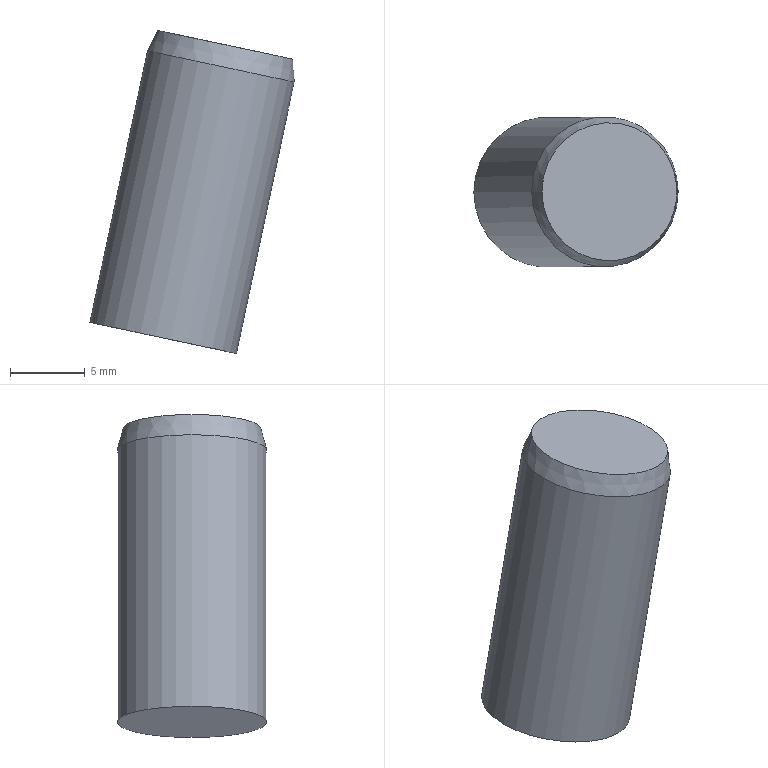Part | STEP file | 8903-XA820 dowel pin (φ8×20) | 1 solid | 4 faces | box 13.634 x 10 x 21.56 mm | volume 1562 mm3 | plane 2 | cone 1 | cylinder 1 | commonest cylinder face diameters 10 x1
STEP:
#1=CARTESIAN_POINT('',(0.,0.,0.));
#2=DIRECTION('',(0.,0.,1.));
#3=DIRECTION('',(1.,0.,0.));
#4=AXIS2_PLACEMENT_3D('',#1,#2,#3);
#5=CARTESIAN_POINT('',(2066.837,-149.5,-389.927));
#6=VERTEX_POINT('',#5);
#7=CARTESIAN_POINT('',(2071.342,-149.5,-390.885));
#8=DIRECTION('',(0.2079,0.,0.9781));
#9=DIRECTION('',(0.9781,0.,-0.2079));
#10=AXIS2_PLACEMENT_3D('',#7,#8,#9);
#11=CIRCLE('',#10,4.607);
#12=CARTESIAN_POINT('',(2069.596,-149.5,-390.514));
#13=DIRECTION('',(0.2079,0.,0.9781));
#14=DIRECTION('',(0.,1.,0.));
#15=AXIS2_PLACEMENT_3D('',#12,#13,#14);
#16=PLANE('',#15);
#17=CARTESIAN_POINT('',(0.,-1.786));
#18=DIRECTION('',(0.,-1.));
#19=AXIS2_PLACEMENT_2D('',#17,#18);
#20=CIRCLE('',#19,4.607);
#21=(GEOMETRIC_REPRESENTATION_CONTEXT(2)PARAMETRIC_REPRESENTATION_CONTEXT()REPRESENTATION_CONTEXT('',''));
#22=DEFINITIONAL_REPRESENTATION('',(#20),#21);
#23=PCURVE('',#16,#22);
#24=CARTESIAN_POINT('',(2071.23,-149.5,-391.414));
#25=DIRECTION('',(-0.2079,0.,-0.9781));
#26=DIRECTION('',(-0.9781,0.,0.2079));
#27=AXIS2_PLACEMENT_3D('',#24,#25,#26);
#28=CONICAL_SURFACE('',#27,4.752,0.2618);
#29=CARTESIAN_POINT('',(9.425,-0.5412));
#30=DIRECTION('',(-1.,0.));
#31=VECTOR('',#30,1.);
#32=LINE('',#29,#31);
#33=(GEOMETRIC_REPRESENTATION_CONTEXT(2)PARAMETRIC_REPRESENTATION_CONTEXT()REPRESENTATION_CONTEXT('',''));
#34=DEFINITIONAL_REPRESENTATION('',(#32),#33);
#35=PCURVE('',#28,#34);
#36=SURFACE_CURVE('',#11,(#23,#35),.PCURVE_S1.);
#37=EDGE_CURVE('',#6,#6,#36,.T.);
#38=ORIENTED_EDGE('',*,*,#37,.T.);
#39=EDGE_LOOP('',(#38));
#40=FACE_BOUND('',#39,.T.);
#41=ADVANCED_FACE('',(#40),#16,.T.);
#42=CARTESIAN_POINT('',(2066.146,-149.5,-391.282));
#43=VERTEX_POINT('',#42);
#44=CARTESIAN_POINT('',(2071.037,-149.5,-392.321));
#45=DIRECTION('',(0.2079,0.,0.9781));
#46=DIRECTION('',(-0.9781,0.,0.2079));
#47=AXIS2_PLACEMENT_3D('',#44,#45,#46);
#48=CIRCLE('',#47,5.);
#49=CARTESIAN_POINT('',(6.283,0.9272));
#50=DIRECTION('',(-1.,0.));
#51=VECTOR('',#50,1.);
#52=LINE('',#49,#51);
#53=(GEOMETRIC_REPRESENTATION_CONTEXT(2)PARAMETRIC_REPRESENTATION_CONTEXT()REPRESENTATION_CONTEXT('',''));
#54=DEFINITIONAL_REPRESENTATION('',(#52),#53);
#55=PCURVE('',#28,#54);
#56=CARTESIAN_POINT('',(2067.247,-149.5,-410.154));
#57=DIRECTION('',(-0.2079,0.,-0.9781));
#58=DIRECTION('',(-0.9781,0.,0.2079));
#59=AXIS2_PLACEMENT_3D('',#56,#57,#58);
#60=CYLINDRICAL_SURFACE('',#59,5.);
#61=CARTESIAN_POINT('',(6.283,-18.232));
#62=DIRECTION('',(-1.,0.));
#63=VECTOR('',#62,1.);
#64=LINE('',#61,#63);
#65=(GEOMETRIC_REPRESENTATION_CONTEXT(2)PARAMETRIC_REPRESENTATION_CONTEXT()REPRESENTATION_CONTEXT('',''));
#66=DEFINITIONAL_REPRESENTATION('',(#64),#65);
#67=PCURVE('',#60,#66);
#68=SURFACE_CURVE('',#48,(#55,#67),.PCURVE_S1.);
#69=EDGE_CURVE('',#43,#43,#68,.T.);
#70=ORIENTED_EDGE('',*,*,#69,.T.);
#71=CARTESIAN_POINT('',(2066.837,-149.5,-389.927));
#72=CARTESIAN_POINT('',(2066.146,-149.5,-391.282));
#73=B_SPLINE_CURVE_WITH_KNOTS('',1,(#71,#72),.UNSPECIFIED.,.F.,.F.,(2,2),(-0.5603,0.9599),.PIECEWISE_BEZIER_KNOTS.);
#74=CARTESIAN_POINT('',(0.,0.));
#75=DIRECTION('',(0.,1.));
#76=VECTOR('',#75,1.);
#77=LINE('',#74,#76);
#78=(GEOMETRIC_REPRESENTATION_CONTEXT(2)PARAMETRIC_REPRESENTATION_CONTEXT()REPRESENTATION_CONTEXT('',''));
#79=DEFINITIONAL_REPRESENTATION('',(#77),#78);
#80=PCURVE('',#28,#79);
#81=CARTESIAN_POINT('',(6.283,0.));
#82=DIRECTION('',(0.,1.));
#83=VECTOR('',#82,1.);
#84=LINE('',#81,#83);
#85=(GEOMETRIC_REPRESENTATION_CONTEXT(2)PARAMETRIC_REPRESENTATION_CONTEXT()REPRESENTATION_CONTEXT('',''));
#86=DEFINITIONAL_REPRESENTATION('',(#84),#85);
#87=PCURVE('',#28,#86);
#88=SEAM_CURVE('',#73,(#80,#87),.PCURVE_S1.);
#89=EDGE_CURVE('',#6,#43,#88,.T.);
#90=ORIENTED_EDGE('',*,*,#89,.F.);
#91=ORIENTED_EDGE('',*,*,#37,.F.);
#92=ORIENTED_EDGE('',*,*,#89,.T.);
#93=EDGE_LOOP('',(#70,#90,#91,#92));
#94=FACE_BOUND('',#93,.T.);
#95=ADVANCED_FACE('',(#94),#28,.T.);
#96=CARTESIAN_POINT('',(2072.075,-149.5,-411.488));
#97=VERTEX_POINT('',#96);
#98=CARTESIAN_POINT('',(2062.294,-149.5,-409.408));
#99=VERTEX_POINT('',#98);
#100=CARTESIAN_POINT('',(2067.184,-149.5,-410.448));
#101=DIRECTION('',(-0.2079,0.,-0.9781));
#102=DIRECTION('',(0.9781,0.,-0.2079));
#103=AXIS2_PLACEMENT_3D('',#100,#101,#102);
#104=CIRCLE('',#103,5.);
#105=CARTESIAN_POINT('',(2007.176,-59.128,-397.693));
#106=DIRECTION('',(0.2079,0.,0.9781));
#107=DIRECTION('',(0.,-1.,0.));
#108=AXIS2_PLACEMENT_3D('',#105,#106,#107);
#109=PLANE('',#108);
#110=CARTESIAN_POINT('',(90.372,66.349));
#111=CARTESIAN_POINT('',(99.032,66.349));
#112=CARTESIAN_POINT('',(94.702,58.849));
#113=CARTESIAN_POINT('',(90.372,51.349));
#114=CARTESIAN_POINT('',(86.042,58.849));
#115=CARTESIAN_POINT('',(81.712,66.349));
#116=CARTESIAN_POINT('',(90.372,66.349));
#117=(BOUNDED_CURVE()B_SPLINE_CURVE(2,(#110,#111,#112,#113,#114,#115,#116),.UNSPECIFIED.,.T.,.F.)B_SPLINE_CURVE_WITH_KNOTS((1,2,2,2,2,1),(-2.094,0.,2.094,4.189,6.283,8.378),.UNSPECIFIED.)CURVE()GEOMETRIC_REPRESENTATION_ITEM()RATIONAL_B_SPLINE_CURVE((1.,0.5,1.,0.5,1.,0.5,1.))REPRESENTATION_ITEM(''));
#118=(GEOMETRIC_REPRESENTATION_CONTEXT(2)PARAMETRIC_REPRESENTATION_CONTEXT()REPRESENTATION_CONTEXT('',''));
#119=DEFINITIONAL_REPRESENTATION('',(#117),#118);
#120=PCURVE('',#109,#119);
#121=CARTESIAN_POINT('',(3.142,0.3));
#122=DIRECTION('',(1.,0.));
#123=VECTOR('',#122,1.);
#124=LINE('',#121,#123);
#125=(GEOMETRIC_REPRESENTATION_CONTEXT(2)PARAMETRIC_REPRESENTATION_CONTEXT()REPRESENTATION_CONTEXT('',''));
#126=DEFINITIONAL_REPRESENTATION('',(#124),#125);
#127=PCURVE('',#60,#126);
#128=SURFACE_CURVE('',#104,(#120,#127),.PCURVE_S1.);
#129=EDGE_CURVE('',#97,#99,#128,.T.);
#130=ORIENTED_EDGE('',*,*,#129,.T.);
#131=CARTESIAN_POINT('',(2067.184,-149.5,-410.448));
#132=DIRECTION('',(-0.2079,0.,-0.9781));
#133=DIRECTION('',(0.9781,0.,-0.2079));
#134=AXIS2_PLACEMENT_3D('',#131,#132,#133);
#135=CIRCLE('',#134,5.);
#136=CARTESIAN_POINT('',(90.372,66.349));
#137=CARTESIAN_POINT('',(99.032,66.349));
#138=CARTESIAN_POINT('',(94.702,58.849));
#139=CARTESIAN_POINT('',(90.372,51.349));
#140=CARTESIAN_POINT('',(86.042,58.849));
#141=CARTESIAN_POINT('',(81.712,66.349));
#142=CARTESIAN_POINT('',(90.372,66.349));
#143=(BOUNDED_CURVE()B_SPLINE_CURVE(2,(#136,#137,#138,#139,#140,#141,#142),.UNSPECIFIED.,.T.,.F.)B_SPLINE_CURVE_WITH_KNOTS((1,2,2,2,2,1),(-2.094,0.,2.094,4.189,6.283,8.378),.UNSPECIFIED.)CURVE()GEOMETRIC_REPRESENTATION_ITEM()RATIONAL_B_SPLINE_CURVE((1.,0.5,1.,0.5,1.,0.5,1.))REPRESENTATION_ITEM(''));
#144=(GEOMETRIC_REPRESENTATION_CONTEXT(2)PARAMETRIC_REPRESENTATION_CONTEXT()REPRESENTATION_CONTEXT('',''));
#145=DEFINITIONAL_REPRESENTATION('',(#143),#144);
#146=PCURVE('',#109,#145);
#147=CARTESIAN_POINT('',(-3.142,0.3));
#148=DIRECTION('',(1.,0.));
#149=VECTOR('',#148,1.);
#150=LINE('',#147,#149);
#151=(GEOMETRIC_REPRESENTATION_CONTEXT(2)PARAMETRIC_REPRESENTATION_CONTEXT()REPRESENTATION_CONTEXT('',''));
#152=DEFINITIONAL_REPRESENTATION('',(#150),#151);
#153=PCURVE('',#60,#152);
#154=SURFACE_CURVE('',#135,(#146,#153),.PCURVE_S1.);
#155=EDGE_CURVE('',#99,#97,#154,.T.);
#156=ORIENTED_EDGE('',*,*,#155,.T.);
#157=EDGE_LOOP('',(#130,#156));
#158=FACE_BOUND('',#157,.T.);
#159=ADVANCED_FACE('',(#158),#109,.F.);
#160=ORIENTED_EDGE('',*,*,#69,.F.);
#161=CARTESIAN_POINT('',(2066.146,-149.5,-391.282));
#162=CARTESIAN_POINT('',(2062.294,-149.5,-409.408));
#163=B_SPLINE_CURVE_WITH_KNOTS('',1,(#161,#162),.UNSPECIFIED.,.F.,.F.,(2,2),(-18.232,0.3),.PIECEWISE_BEZIER_KNOTS.);
#164=CARTESIAN_POINT('',(6.283,0.));
#165=DIRECTION('',(0.,1.));
#166=VECTOR('',#165,1.);
#167=LINE('',#164,#166);
#168=(GEOMETRIC_REPRESENTATION_CONTEXT(2)PARAMETRIC_REPRESENTATION_CONTEXT()REPRESENTATION_CONTEXT('',''));
#169=DEFINITIONAL_REPRESENTATION('',(#167),#168);
#170=PCURVE('',#60,#169);
#171=CARTESIAN_POINT('',(0.,0.));
#172=DIRECTION('',(0.,1.));
#173=VECTOR('',#172,1.);
#174=LINE('',#171,#173);
#175=(GEOMETRIC_REPRESENTATION_CONTEXT(2)PARAMETRIC_REPRESENTATION_CONTEXT()REPRESENTATION_CONTEXT('',''));
#176=DEFINITIONAL_REPRESENTATION('',(#174),#175);
#177=PCURVE('',#60,#176);
#178=SEAM_CURVE('',#163,(#170,#177),.PCURVE_S1.);
#179=EDGE_CURVE('',#43,#99,#178,.T.);
#180=ORIENTED_EDGE('',*,*,#179,.T.);
#181=ORIENTED_EDGE('',*,*,#129,.F.);
#182=ORIENTED_EDGE('',*,*,#155,.F.);
#183=ORIENTED_EDGE('',*,*,#179,.F.);
#184=EDGE_LOOP('',(#160,#180,#181,#182,#183));
#185=FACE_BOUND('',#184,.T.);
#186=ADVANCED_FACE('',(#185),#60,.T.);
#187=CLOSED_SHELL('',(#41,#95,#159,#186));
#188=MANIFOLD_SOLID_BREP('',#187);
#189=(LENGTH_UNIT()NAMED_UNIT(*)SI_UNIT(.MILLI.,.METRE.));
#190=UNCERTAINTY_MEASURE_WITH_UNIT(LENGTH_MEASURE(0.000005),#189,'','');
#191=(NAMED_UNIT(*)PLANE_ANGLE_UNIT()SI_UNIT($,.RADIAN.));
#192=(NAMED_UNIT(*)SI_UNIT($,.STERADIAN.)SOLID_ANGLE_UNIT());
#193=(GEOMETRIC_REPRESENTATION_CONTEXT(3)GLOBAL_UNCERTAINTY_ASSIGNED_CONTEXT((#190))GLOBAL_UNIT_ASSIGNED_CONTEXT((#189,#191,#192))REPRESENTATION_CONTEXT('',''));
#194=ADVANCED_BREP_SHAPE_REPRESENTATION('',(#4,#188),#193);